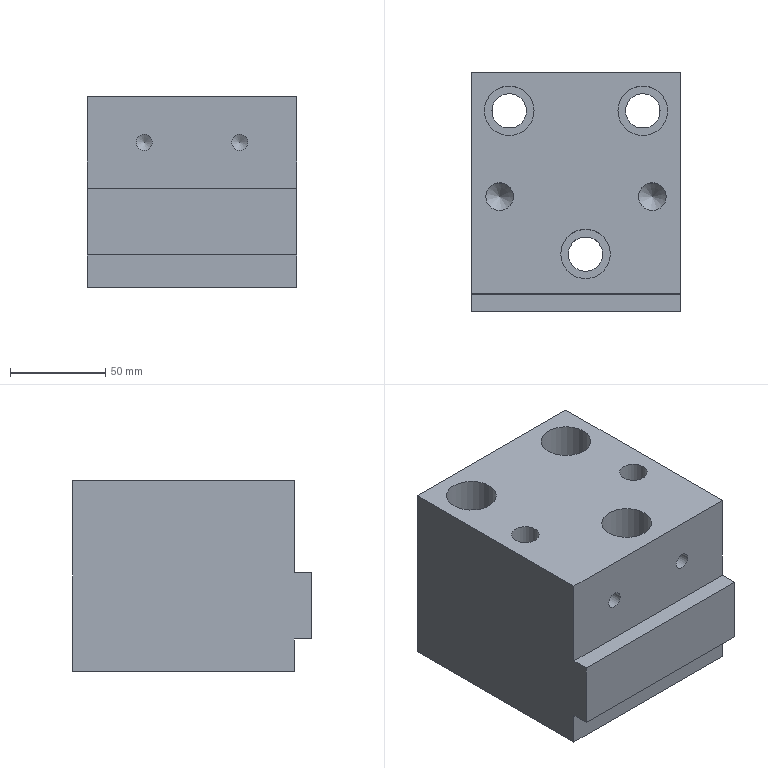Part | STEP file | lll_id4734_x_t | 1 solid | 27 faces | box 110 x 125 x 100 mm | volume 1168907 mm3 | plane 13 | cylinder 10 | cone 4 | commonest cylinder face diameters 18.009 x3 26.008 x3 8.5 x2 14.506 x2
STEP:
#1=CARTESIAN_POINT('',(1322.592,417.359,5.));
#2=VERTEX_POINT('',#1);
#3=CARTESIAN_POINT('',(1315.339,417.359,5.));
#4=DIRECTION('',(0.,0.,-1.));
#5=DIRECTION('',(1.,0.,0.));
#6=AXIS2_PLACEMENT_3D('',#3,#4,#5);
#7=CIRCLE('',#6,7.253);
#8=EDGE_CURVE('',#2,#2,#7,.T.);
#9=ORIENTED_EDGE('',*,*,#8,.T.);
#10=EDGE_LOOP('',(#9));
#11=FACE_BOUND('',#10,.T.);
#12=CARTESIAN_POINT('',(1402.592,417.359,5.));
#13=VERTEX_POINT('',#12);
#14=CARTESIAN_POINT('',(1395.339,417.359,5.));
#15=DIRECTION('',(0.,0.,-1.));
#16=DIRECTION('',(1.,0.,0.));
#17=AXIS2_PLACEMENT_3D('',#14,#15,#16);
#18=CIRCLE('',#17,7.253);
#19=EDGE_CURVE('',#13,#13,#18,.T.);
#20=ORIENTED_EDGE('',*,*,#19,.T.);
#21=EDGE_LOOP('',(#20));
#22=FACE_BOUND('',#21,.T.);
#23=CARTESIAN_POINT('',(1300.339,366.359,5.));
#24=VERTEX_POINT('',#23);
#25=CARTESIAN_POINT('',(1410.339,366.359,5.));
#26=VERTEX_POINT('',#25);
#27=CARTESIAN_POINT('',(-3297.001,366.359,5.));
#28=DIRECTION('',(1.,0.,0.));
#29=VECTOR('',#28,1.);
#30=LINE('',#27,#29);
#31=EDGE_CURVE('',#24,#26,#30,.T.);
#32=ORIENTED_EDGE('',*,*,#31,.T.);
#33=CARTESIAN_POINT('',(1410.339,482.359,5.));
#34=VERTEX_POINT('',#33);
#35=CARTESIAN_POINT('',(1410.339,382.359,5.));
#36=DIRECTION('',(0.,-1.,0.));
#37=VECTOR('',#36,1.);
#38=LINE('',#35,#37);
#39=EDGE_CURVE('',#34,#26,#38,.T.);
#40=ORIENTED_EDGE('',*,*,#39,.F.);
#41=CARTESIAN_POINT('',(1300.339,482.359,5.));
#42=VERTEX_POINT('',#41);
#43=CARTESIAN_POINT('',(1308.588,482.359,5.));
#44=DIRECTION('',(-1.,0.,0.));
#45=VECTOR('',#44,1.);
#46=LINE('',#43,#45);
#47=EDGE_CURVE('',#34,#42,#46,.T.);
#48=ORIENTED_EDGE('',*,*,#47,.T.);
#49=CARTESIAN_POINT('',(1300.339,382.359,5.));
#50=DIRECTION('',(0.,1.,0.));
#51=VECTOR('',#50,1.);
#52=LINE('',#49,#51);
#53=EDGE_CURVE('',#24,#42,#52,.T.);
#54=ORIENTED_EDGE('',*,*,#53,.F.);
#55=EDGE_LOOP('',(#32,#40,#48,#54));
#56=FACE_BOUND('',#55,.T.);
#57=CARTESIAN_POINT('',(1377.335,462.359,5.));
#58=VERTEX_POINT('',#57);
#59=CARTESIAN_POINT('',(1390.339,462.359,5.));
#60=DIRECTION('',(0.,0.,-1.));
#61=DIRECTION('',(-1.,0.,0.));
#62=AXIS2_PLACEMENT_3D('',#59,#60,#61);
#63=CIRCLE('',#62,13.004);
#64=EDGE_CURVE('',#58,#58,#63,.T.);
#65=ORIENTED_EDGE('',*,*,#64,.T.);
#66=EDGE_LOOP('',(#65));
#67=FACE_BOUND('',#66,.T.);
#68=CARTESIAN_POINT('',(1307.335,462.359,5.));
#69=VERTEX_POINT('',#68);
#70=CARTESIAN_POINT('',(1320.339,462.359,5.));
#71=DIRECTION('',(0.,0.,-1.));
#72=DIRECTION('',(-1.,0.,0.));
#73=AXIS2_PLACEMENT_3D('',#70,#71,#72);
#74=CIRCLE('',#73,13.004);
#75=EDGE_CURVE('',#69,#69,#74,.T.);
#76=ORIENTED_EDGE('',*,*,#75,.T.);
#77=EDGE_LOOP('',(#76));
#78=FACE_BOUND('',#77,.T.);
#79=CARTESIAN_POINT('',(1373.343,387.359,5.));
#80=VERTEX_POINT('',#79);
#81=CARTESIAN_POINT('',(1360.339,387.359,5.));
#82=DIRECTION('',(0.,0.,1.));
#83=DIRECTION('',(1.,0.,0.));
#84=AXIS2_PLACEMENT_3D('',#81,#82,#83);
#85=CIRCLE('',#84,13.004);
#86=EDGE_CURVE('',#80,#80,#85,.T.);
#87=ORIENTED_EDGE('',*,*,#86,.F.);
#88=EDGE_LOOP('',(#87));
#89=FACE_BOUND('',#88,.T.);
#90=CARTESIAN_POINT('',(1308.588,382.359,5.));
#91=DIRECTION('',(0.,0.,-1.));
#92=DIRECTION('',(1.,0.,0.));
#93=AXIS2_PLACEMENT_3D('',#90,#91,#92);
#94=PLANE('',#93);
#95=ADVANCED_FACE('',(#11,#22,#56,#67,#78,#89),#94,.F.);
#96=CARTESIAN_POINT('',(1330.339,366.359,-23.25));
#97=VERTEX_POINT('',#96);
#98=CARTESIAN_POINT('',(1330.339,366.359,-19.));
#99=DIRECTION('',(0.,-1.,0.));
#100=DIRECTION('',(0.,0.,-1.));
#101=AXIS2_PLACEMENT_3D('',#98,#99,#100);
#102=CIRCLE('',#101,4.25);
#103=EDGE_CURVE('',#97,#97,#102,.T.);
#104=ORIENTED_EDGE('',*,*,#103,.F.);
#105=EDGE_LOOP('',(#104));
#106=FACE_BOUND('',#105,.T.);
#107=CARTESIAN_POINT('',(1380.339,366.359,-23.25));
#108=VERTEX_POINT('',#107);
#109=CARTESIAN_POINT('',(1380.339,366.359,-19.));
#110=DIRECTION('',(0.,-1.,0.));
#111=DIRECTION('',(0.,0.,-1.));
#112=AXIS2_PLACEMENT_3D('',#109,#110,#111);
#113=CIRCLE('',#112,4.25);
#114=EDGE_CURVE('',#108,#108,#113,.T.);
#115=ORIENTED_EDGE('',*,*,#114,.F.);
#116=EDGE_LOOP('',(#115));
#117=FACE_BOUND('',#116,.T.);
#118=CARTESIAN_POINT('',(1300.339,366.359,-43.));
#119=VERTEX_POINT('',#118);
#120=CARTESIAN_POINT('',(1410.339,366.359,-43.));
#121=VERTEX_POINT('',#120);
#122=CARTESIAN_POINT('',(1305.339,366.359,-43.));
#123=DIRECTION('',(1.,0.,0.));
#124=VECTOR('',#123,1.);
#125=LINE('',#122,#124);
#126=EDGE_CURVE('',#119,#121,#125,.T.);
#127=ORIENTED_EDGE('',*,*,#126,.T.);
#128=CARTESIAN_POINT('',(1410.339,366.359,-35.));
#129=DIRECTION('',(0.,0.,1.));
#130=VECTOR('',#129,1.);
#131=LINE('',#128,#130);
#132=EDGE_CURVE('',#121,#26,#131,.T.);
#133=ORIENTED_EDGE('',*,*,#132,.T.);
#134=ORIENTED_EDGE('',*,*,#31,.F.);
#135=CARTESIAN_POINT('',(1300.339,366.359,-625.));
#136=DIRECTION('',(0.,0.,-1.));
#137=VECTOR('',#136,1.);
#138=LINE('',#135,#137);
#139=EDGE_CURVE('',#24,#119,#138,.T.);
#140=ORIENTED_EDGE('',*,*,#139,.T.);
#141=EDGE_LOOP('',(#127,#133,#134,#140));
#142=FACE_BOUND('',#141,.T.);
#143=CARTESIAN_POINT('',(-3297.001,366.359,-625.));
#144=DIRECTION('',(0.,-1.,0.));
#145=DIRECTION('',(0.,0.,1.));
#146=AXIS2_PLACEMENT_3D('',#143,#144,#145);
#147=PLANE('',#146);
#148=ADVANCED_FACE('',(#106,#117,#142),#147,.T.);
#149=CARTESIAN_POINT('',(1300.339,482.359,-95.));
#150=VERTEX_POINT('',#149);
#151=CARTESIAN_POINT('',(1300.339,482.359,-650.));
#152=DIRECTION('',(0.,0.,-1.));
#153=VECTOR('',#152,1.);
#154=LINE('',#151,#153);
#155=EDGE_CURVE('',#42,#150,#154,.T.);
#156=ORIENTED_EDGE('',*,*,#155,.T.);
#157=CARTESIAN_POINT('',(1300.339,366.359,-95.));
#158=VERTEX_POINT('',#157);
#159=CARTESIAN_POINT('',(1300.339,407.359,-95.));
#160=DIRECTION('',(0.,-1.,0.));
#161=VECTOR('',#160,1.);
#162=LINE('',#159,#161);
#163=EDGE_CURVE('',#150,#158,#162,.T.);
#164=ORIENTED_EDGE('',*,*,#163,.T.);
#165=CARTESIAN_POINT('',(1300.339,366.359,-78.));
#166=VERTEX_POINT('',#165);
#167=CARTESIAN_POINT('',(1300.339,366.359,-625.));
#168=DIRECTION('',(0.,0.,-1.));
#169=VECTOR('',#168,1.);
#170=LINE('',#167,#169);
#171=EDGE_CURVE('',#166,#158,#170,.T.);
#172=ORIENTED_EDGE('',*,*,#171,.F.);
#173=CARTESIAN_POINT('',(1300.339,357.359,-78.));
#174=VERTEX_POINT('',#173);
#175=CARTESIAN_POINT('',(1300.339,407.359,-78.));
#176=DIRECTION('',(0.,-1.,0.));
#177=VECTOR('',#176,1.);
#178=LINE('',#175,#177);
#179=EDGE_CURVE('',#166,#174,#178,.T.);
#180=ORIENTED_EDGE('',*,*,#179,.T.);
#181=CARTESIAN_POINT('',(1300.339,357.359,-43.));
#182=VERTEX_POINT('',#181);
#183=CARTESIAN_POINT('',(1300.339,357.359,72.5));
#184=DIRECTION('',(0.,0.,-1.));
#185=VECTOR('',#184,1.);
#186=LINE('',#183,#185);
#187=EDGE_CURVE('',#182,#174,#186,.T.);
#188=ORIENTED_EDGE('',*,*,#187,.F.);
#189=CARTESIAN_POINT('',(1300.339,397.359,-43.));
#190=DIRECTION('',(0.,-1.,0.));
#191=VECTOR('',#190,1.);
#192=LINE('',#189,#191);
#193=EDGE_CURVE('',#119,#182,#192,.T.);
#194=ORIENTED_EDGE('',*,*,#193,.F.);
#195=ORIENTED_EDGE('',*,*,#139,.F.);
#196=ORIENTED_EDGE('',*,*,#53,.T.);
#197=EDGE_LOOP('',(#156,#164,#172,#180,#188,#194,#195,#196));
#198=FACE_OUTER_BOUND('',#197,.T.);
#199=CARTESIAN_POINT('',(1300.339,407.359,72.5));
#200=DIRECTION('',(-1.,0.,0.));
#201=DIRECTION('',(0.,0.,-1.));
#202=AXIS2_PLACEMENT_3D('',#199,#200,#201);
#203=PLANE('',#202);
#204=ADVANCED_FACE('',(#198),#203,.T.);
#205=CARTESIAN_POINT('',(1410.339,357.359,-78.));
#206=VERTEX_POINT('',#205);
#207=CARTESIAN_POINT('',(-3297.001,357.359,-78.));
#208=DIRECTION('',(-1.,0.,0.));
#209=VECTOR('',#208,1.);
#210=LINE('',#207,#209);
#211=EDGE_CURVE('',#206,#174,#210,.T.);
#212=ORIENTED_EDGE('',*,*,#211,.F.);
#213=CARTESIAN_POINT('',(1410.339,357.359,-43.));
#214=VERTEX_POINT('',#213);
#215=CARTESIAN_POINT('',(1410.339,357.359,-60.));
#216=DIRECTION('',(0.,0.,1.));
#217=VECTOR('',#216,1.);
#218=LINE('',#215,#217);
#219=EDGE_CURVE('',#206,#214,#218,.T.);
#220=ORIENTED_EDGE('',*,*,#219,.T.);
#221=CARTESIAN_POINT('',(-3297.001,357.359,-43.));
#222=DIRECTION('',(-1.,0.,0.));
#223=VECTOR('',#222,1.);
#224=LINE('',#221,#223);
#225=EDGE_CURVE('',#214,#182,#224,.T.);
#226=ORIENTED_EDGE('',*,*,#225,.T.);
#227=ORIENTED_EDGE('',*,*,#187,.T.);
#228=EDGE_LOOP('',(#212,#220,#226,#227));
#229=FACE_OUTER_BOUND('',#228,.T.);
#230=CARTESIAN_POINT('',(-3297.001,357.359,-650.));
#231=DIRECTION('',(0.,-1.,0.));
#232=DIRECTION('',(0.,0.,1.));
#233=AXIS2_PLACEMENT_3D('',#230,#231,#232);
#234=PLANE('',#233);
#235=ADVANCED_FACE('',(#229),#234,.T.);
#236=CARTESIAN_POINT('',(1410.339,482.359,-95.));
#237=VERTEX_POINT('',#236);
#238=CARTESIAN_POINT('',(1410.339,482.359,-650.));
#239=DIRECTION('',(0.,0.,-1.));
#240=VECTOR('',#239,1.);
#241=LINE('',#238,#240);
#242=EDGE_CURVE('',#34,#237,#241,.T.);
#243=ORIENTED_EDGE('',*,*,#242,.T.);
#244=CARTESIAN_POINT('',(-3297.001,482.359,-95.));
#245=DIRECTION('',(1.,0.,0.));
#246=VECTOR('',#245,1.);
#247=LINE('',#244,#246);
#248=EDGE_CURVE('',#150,#237,#247,.T.);
#249=ORIENTED_EDGE('',*,*,#248,.F.);
#250=ORIENTED_EDGE('',*,*,#155,.F.);
#251=ORIENTED_EDGE('',*,*,#47,.F.);
#252=EDGE_LOOP('',(#243,#249,#250,#251));
#253=FACE_OUTER_BOUND('',#252,.T.);
#254=CARTESIAN_POINT('',(-3297.001,482.359,-650.));
#255=DIRECTION('',(0.,-1.,0.));
#256=DIRECTION('',(0.,0.,1.));
#257=AXIS2_PLACEMENT_3D('',#254,#255,#256);
#258=PLANE('',#257);
#259=ADVANCED_FACE('',(#253),#258,.F.);
#260=ORIENTED_EDGE('',*,*,#219,.F.);
#261=CARTESIAN_POINT('',(1410.339,366.359,-78.));
#262=VERTEX_POINT('',#261);
#263=CARTESIAN_POINT('',(1410.339,382.359,-78.));
#264=DIRECTION('',(0.,-1.,0.));
#265=VECTOR('',#264,1.);
#266=LINE('',#263,#265);
#267=EDGE_CURVE('',#262,#206,#266,.T.);
#268=ORIENTED_EDGE('',*,*,#267,.F.);
#269=CARTESIAN_POINT('',(1410.339,366.359,-95.));
#270=VERTEX_POINT('',#269);
#271=CARTESIAN_POINT('',(1410.339,366.359,-60.));
#272=DIRECTION('',(0.,0.,1.));
#273=VECTOR('',#272,1.);
#274=LINE('',#271,#273);
#275=EDGE_CURVE('',#270,#262,#274,.T.);
#276=ORIENTED_EDGE('',*,*,#275,.F.);
#277=CARTESIAN_POINT('',(1410.339,233.52,-95.));
#278=DIRECTION('',(0.,1.,0.));
#279=VECTOR('',#278,1.);
#280=LINE('',#277,#279);
#281=EDGE_CURVE('',#270,#237,#280,.T.);
#282=ORIENTED_EDGE('',*,*,#281,.T.);
#283=ORIENTED_EDGE('',*,*,#242,.F.);
#284=ORIENTED_EDGE('',*,*,#39,.T.);
#285=ORIENTED_EDGE('',*,*,#132,.F.);
#286=CARTESIAN_POINT('',(1410.339,382.359,-43.));
#287=DIRECTION('',(0.,1.,0.));
#288=VECTOR('',#287,1.);
#289=LINE('',#286,#288);
#290=EDGE_CURVE('',#214,#121,#289,.T.);
#291=ORIENTED_EDGE('',*,*,#290,.F.);
#292=EDGE_LOOP('',(#260,#268,#276,#282,#283,#284,#285,#291));
#293=FACE_OUTER_BOUND('',#292,.T.);
#294=CARTESIAN_POINT('',(1410.339,382.359,-60.));
#295=DIRECTION('',(-1.,0.,0.));
#296=DIRECTION('',(0.,0.,-1.));
#297=AXIS2_PLACEMENT_3D('',#294,#295,#296);
#298=PLANE('',#297);
#299=ADVANCED_FACE('',(#293),#298,.F.);
#300=ORIENTED_EDGE('',*,*,#126,.F.);
#301=ORIENTED_EDGE('',*,*,#193,.T.);
#302=ORIENTED_EDGE('',*,*,#225,.F.);
#303=ORIENTED_EDGE('',*,*,#290,.T.);
#304=EDGE_LOOP('',(#300,#301,#302,#303));
#305=FACE_OUTER_BOUND('',#304,.T.);
#306=CARTESIAN_POINT('',(1305.339,397.359,-43.));
#307=DIRECTION('',(0.,0.,1.));
#308=DIRECTION('',(-1.,0.,0.));
#309=AXIS2_PLACEMENT_3D('',#306,#307,#308);
#310=PLANE('',#309);
#311=ADVANCED_FACE('',(#305),#310,.T.);
#312=CARTESIAN_POINT('',(1399.344,462.359,-55.));
#313=VERTEX_POINT('',#312);
#314=CARTESIAN_POINT('',(1390.339,462.359,-55.));
#315=DIRECTION('',(0.,0.,-1.));
#316=DIRECTION('',(1.,0.,0.));
#317=AXIS2_PLACEMENT_3D('',#314,#315,#316);
#318=CIRCLE('',#317,9.005);
#319=EDGE_CURVE('',#313,#313,#318,.T.);
#320=ORIENTED_EDGE('',*,*,#319,.F.);
#321=EDGE_LOOP('',(#320));
#322=FACE_BOUND('',#321,.T.);
#323=CARTESIAN_POINT('',(1399.344,462.359,-95.));
#324=VERTEX_POINT('',#323);
#325=CARTESIAN_POINT('',(1390.339,462.359,-95.));
#326=DIRECTION('',(0.,0.,-1.));
#327=DIRECTION('',(1.,0.,0.));
#328=AXIS2_PLACEMENT_3D('',#325,#326,#327);
#329=CIRCLE('',#328,9.005);
#330=EDGE_CURVE('',#324,#324,#329,.T.);
#331=ORIENTED_EDGE('',*,*,#330,.T.);
#332=EDGE_LOOP('',(#331));
#333=FACE_BOUND('',#332,.T.);
#334=CARTESIAN_POINT('',(1390.339,462.359,-18.));
#335=DIRECTION('',(0.,0.,-1.));
#336=DIRECTION('',(-1.,0.,0.));
#337=AXIS2_PLACEMENT_3D('',#334,#335,#336);
#338=CYLINDRICAL_SURFACE('',#337,9.005);
#339=ADVANCED_FACE('',(#322,#333),#338,.F.);
#340=ORIENTED_EDGE('',*,*,#319,.T.);
#341=EDGE_LOOP('',(#340));
#342=FACE_BOUND('',#341,.T.);
#343=CARTESIAN_POINT('',(1377.335,462.359,-55.));
#344=VERTEX_POINT('',#343);
#345=CARTESIAN_POINT('',(1390.339,462.359,-55.));
#346=DIRECTION('',(0.,0.,-1.));
#347=DIRECTION('',(-1.,0.,0.));
#348=AXIS2_PLACEMENT_3D('',#345,#346,#347);
#349=CIRCLE('',#348,13.004);
#350=EDGE_CURVE('',#344,#344,#349,.T.);
#351=ORIENTED_EDGE('',*,*,#350,.F.);
#352=EDGE_LOOP('',(#351));
#353=FACE_BOUND('',#352,.T.);
#354=CARTESIAN_POINT('',(1390.339,462.359,-55.));
#355=DIRECTION('',(0.,0.,-1.));
#356=DIRECTION('',(1.,0.,0.));
#357=AXIS2_PLACEMENT_3D('',#354,#355,#356);
#358=PLANE('',#357);
#359=ADVANCED_FACE('',(#342,#353),#358,.F.);
#360=ORIENTED_EDGE('',*,*,#350,.T.);
#361=EDGE_LOOP('',(#360));
#362=FACE_BOUND('',#361,.T.);
#363=ORIENTED_EDGE('',*,*,#64,.F.);
#364=EDGE_LOOP('',(#363));
#365=FACE_BOUND('',#364,.T.);
#366=CARTESIAN_POINT('',(1390.339,462.359,5.));
#367=DIRECTION('',(0.,0.,-1.));
#368=DIRECTION('',(-1.,0.,0.));
#369=AXIS2_PLACEMENT_3D('',#366,#367,#368);
#370=CYLINDRICAL_SURFACE('',#369,13.004);
#371=ADVANCED_FACE('',(#362,#365),#370,.F.);
#372=CARTESIAN_POINT('',(1329.344,462.359,-55.));
#373=VERTEX_POINT('',#372);
#374=CARTESIAN_POINT('',(1320.339,462.359,-55.));
#375=DIRECTION('',(0.,0.,-1.));
#376=DIRECTION('',(0.,1.,0.));
#377=AXIS2_PLACEMENT_3D('',#374,#375,#376);
#378=CIRCLE('',#377,9.005);
#379=EDGE_CURVE('',#373,#373,#378,.T.);
#380=ORIENTED_EDGE('',*,*,#379,.F.);
#381=EDGE_LOOP('',(#380));
#382=FACE_BOUND('',#381,.T.);
#383=CARTESIAN_POINT('',(1329.344,462.359,-95.));
#384=VERTEX_POINT('',#383);
#385=CARTESIAN_POINT('',(1320.339,462.359,-95.));
#386=DIRECTION('',(0.,0.,-1.));
#387=DIRECTION('',(1.,0.,0.));
#388=AXIS2_PLACEMENT_3D('',#385,#386,#387);
#389=CIRCLE('',#388,9.005);
#390=EDGE_CURVE('',#384,#384,#389,.T.);
#391=ORIENTED_EDGE('',*,*,#390,.T.);
#392=EDGE_LOOP('',(#391));
#393=FACE_BOUND('',#392,.T.);
#394=CARTESIAN_POINT('',(1320.339,462.359,-18.));
#395=DIRECTION('',(0.,0.,-1.));
#396=DIRECTION('',(-1.,0.,0.));
#397=AXIS2_PLACEMENT_3D('',#394,#395,#396);
#398=CYLINDRICAL_SURFACE('',#397,9.005);
#399=ADVANCED_FACE('',(#382,#393),#398,.F.);
#400=ORIENTED_EDGE('',*,*,#379,.T.);
#401=EDGE_LOOP('',(#400));
#402=FACE_BOUND('',#401,.T.);
#403=CARTESIAN_POINT('',(1307.335,462.359,-55.));
#404=VERTEX_POINT('',#403);
#405=CARTESIAN_POINT('',(1320.339,462.359,-55.));
#406=DIRECTION('',(0.,0.,-1.));
#407=DIRECTION('',(0.,1.,0.));
#408=AXIS2_PLACEMENT_3D('',#405,#406,#407);
#409=CIRCLE('',#408,13.004);
#410=EDGE_CURVE('',#404,#404,#409,.T.);
#411=ORIENTED_EDGE('',*,*,#410,.F.);
#412=EDGE_LOOP('',(#411));
#413=FACE_BOUND('',#412,.T.);
#414=CARTESIAN_POINT('',(1320.339,462.359,-55.));
#415=DIRECTION('',(0.,0.,-1.));
#416=DIRECTION('',(1.,0.,0.));
#417=AXIS2_PLACEMENT_3D('',#414,#415,#416);
#418=PLANE('',#417);
#419=ADVANCED_FACE('',(#402,#413),#418,.F.);
#420=ORIENTED_EDGE('',*,*,#410,.T.);
#421=EDGE_LOOP('',(#420));
#422=FACE_BOUND('',#421,.T.);
#423=ORIENTED_EDGE('',*,*,#75,.F.);
#424=EDGE_LOOP('',(#423));
#425=FACE_BOUND('',#424,.T.);
#426=CARTESIAN_POINT('',(1320.339,462.359,5.));
#427=DIRECTION('',(0.,0.,-1.));
#428=DIRECTION('',(-1.,0.,0.));
#429=AXIS2_PLACEMENT_3D('',#426,#427,#428);
#430=CYLINDRICAL_SURFACE('',#429,13.004);
#431=ADVANCED_FACE('',(#422,#425),#430,.F.);
#432=CARTESIAN_POINT('',(1351.335,387.359,-55.));
#433=VERTEX_POINT('',#432);
#434=CARTESIAN_POINT('',(1360.339,387.359,-55.));
#435=DIRECTION('',(0.,0.,1.));
#436=DIRECTION('',(-1.,0.,0.));
#437=AXIS2_PLACEMENT_3D('',#434,#435,#436);
#438=CIRCLE('',#437,9.005);
#439=EDGE_CURVE('',#433,#433,#438,.T.);
#440=ORIENTED_EDGE('',*,*,#439,.T.);
#441=EDGE_LOOP('',(#440));
#442=FACE_BOUND('',#441,.T.);
#443=CARTESIAN_POINT('',(1369.344,387.359,-95.));
#444=VERTEX_POINT('',#443);
#445=CARTESIAN_POINT('',(1360.339,387.359,-95.));
#446=DIRECTION('',(0.,0.,-1.));
#447=DIRECTION('',(1.,0.,0.));
#448=AXIS2_PLACEMENT_3D('',#445,#446,#447);
#449=CIRCLE('',#448,9.005);
#450=EDGE_CURVE('',#444,#444,#449,.T.);
#451=ORIENTED_EDGE('',*,*,#450,.T.);
#452=EDGE_LOOP('',(#451));
#453=FACE_BOUND('',#452,.T.);
#454=CARTESIAN_POINT('',(1360.339,387.359,-18.));
#455=DIRECTION('',(0.,0.,-1.));
#456=DIRECTION('',(1.,0.,0.));
#457=AXIS2_PLACEMENT_3D('',#454,#455,#456);
#458=CYLINDRICAL_SURFACE('',#457,9.005);
#459=ADVANCED_FACE('',(#442,#453),#458,.F.);
#460=ORIENTED_EDGE('',*,*,#439,.F.);
#461=EDGE_LOOP('',(#460));
#462=FACE_BOUND('',#461,.T.);
#463=CARTESIAN_POINT('',(1373.343,387.359,-55.));
#464=VERTEX_POINT('',#463);
#465=CARTESIAN_POINT('',(1360.339,387.359,-55.));
#466=DIRECTION('',(0.,0.,1.));
#467=DIRECTION('',(1.,0.,0.));
#468=AXIS2_PLACEMENT_3D('',#465,#466,#467);
#469=CIRCLE('',#468,13.004);
#470=EDGE_CURVE('',#464,#464,#469,.T.);
#471=ORIENTED_EDGE('',*,*,#470,.T.);
#472=EDGE_LOOP('',(#471));
#473=FACE_BOUND('',#472,.T.);
#474=CARTESIAN_POINT('',(1360.339,387.359,-55.));
#475=DIRECTION('',(0.,0.,-1.));
#476=DIRECTION('',(-1.,0.,0.));
#477=AXIS2_PLACEMENT_3D('',#474,#475,#476);
#478=PLANE('',#477);
#479=ADVANCED_FACE('',(#462,#473),#478,.F.);
#480=ORIENTED_EDGE('',*,*,#470,.F.);
#481=EDGE_LOOP('',(#480));
#482=FACE_BOUND('',#481,.T.);
#483=ORIENTED_EDGE('',*,*,#86,.T.);
#484=EDGE_LOOP('',(#483));
#485=FACE_BOUND('',#484,.T.);
#486=CARTESIAN_POINT('',(1360.339,387.359,5.));
#487=DIRECTION('',(0.,0.,-1.));
#488=DIRECTION('',(1.,0.,0.));
#489=AXIS2_PLACEMENT_3D('',#486,#487,#488);
#490=CYLINDRICAL_SURFACE('',#489,13.004);
#491=ADVANCED_FACE('',(#482,#485),#490,.F.);
#492=CARTESIAN_POINT('',(1402.592,417.359,-30.753));
#493=VERTEX_POINT('',#492);
#494=CARTESIAN_POINT('',(1395.339,417.359,-30.753));
#495=DIRECTION('',(0.,0.,-1.));
#496=DIRECTION('',(1.,0.,0.));
#497=AXIS2_PLACEMENT_3D('',#494,#495,#496);
#498=CIRCLE('',#497,7.253);
#499=EDGE_CURVE('',#493,#493,#498,.T.);
#500=ORIENTED_EDGE('',*,*,#499,.T.);
#501=EDGE_LOOP('',(#500));
#502=FACE_BOUND('',#501,.T.);
#503=ORIENTED_EDGE('',*,*,#19,.F.);
#504=EDGE_LOOP('',(#503));
#505=FACE_BOUND('',#504,.T.);
#506=CARTESIAN_POINT('',(1395.339,417.359,7.));
#507=DIRECTION('',(0.,0.,-1.));
#508=DIRECTION('',(-1.,0.,0.));
#509=AXIS2_PLACEMENT_3D('',#506,#507,#508);
#510=CYLINDRICAL_SURFACE('',#509,7.253);
#511=ADVANCED_FACE('',(#502,#505),#510,.F.);
#512=CARTESIAN_POINT('',(1395.339,417.359,-38.006));
#513=VERTEX_POINT('',#512);
#514=VERTEX_LOOP('',#513);
#515=FACE_BOUND('',#514,.T.);
#516=ORIENTED_EDGE('',*,*,#499,.F.);
#517=EDGE_LOOP('',(#516));
#518=FACE_BOUND('',#517,.T.);
#519=CARTESIAN_POINT('',(1395.339,417.359,-30.753));
#520=DIRECTION('',(0.,0.,1.));
#521=DIRECTION('',(-1.,0.,0.));
#522=AXIS2_PLACEMENT_3D('',#519,#520,#521);
#523=CONICAL_SURFACE('',#522,7.253,45.);
#524=ADVANCED_FACE('',(#515,#518),#523,.F.);
#525=CARTESIAN_POINT('',(1308.086,417.359,-30.753));
#526=VERTEX_POINT('',#525);
#527=CARTESIAN_POINT('',(1315.339,417.359,-30.753));
#528=DIRECTION('',(0.,0.,1.));
#529=DIRECTION('',(-1.,0.,0.));
#530=AXIS2_PLACEMENT_3D('',#527,#528,#529);
#531=CIRCLE('',#530,7.253);
#532=EDGE_CURVE('',#526,#526,#531,.T.);
#533=ORIENTED_EDGE('',*,*,#532,.F.);
#534=EDGE_LOOP('',(#533));
#535=FACE_BOUND('',#534,.T.);
#536=ORIENTED_EDGE('',*,*,#8,.F.);
#537=EDGE_LOOP('',(#536));
#538=FACE_BOUND('',#537,.T.);
#539=CARTESIAN_POINT('',(1315.339,417.359,7.));
#540=DIRECTION('',(0.,0.,-1.));
#541=DIRECTION('',(1.,0.,0.));
#542=AXIS2_PLACEMENT_3D('',#539,#540,#541);
#543=CYLINDRICAL_SURFACE('',#542,7.253);
#544=ADVANCED_FACE('',(#535,#538),#543,.F.);
#545=CARTESIAN_POINT('',(1315.339,417.359,-38.006));
#546=VERTEX_POINT('',#545);
#547=VERTEX_LOOP('',#546);
#548=FACE_BOUND('',#547,.T.);
#549=ORIENTED_EDGE('',*,*,#532,.T.);
#550=EDGE_LOOP('',(#549));
#551=FACE_BOUND('',#550,.T.);
#552=CARTESIAN_POINT('',(1315.339,417.359,-30.753));
#553=DIRECTION('',(0.,0.,1.));
#554=DIRECTION('',(1.,0.,0.));
#555=AXIS2_PLACEMENT_3D('',#552,#553,#554);
#556=CONICAL_SURFACE('',#555,7.253,45.);
#557=ADVANCED_FACE('',(#548,#551),#556,.F.);
#558=CARTESIAN_POINT('',(1380.339,396.359,-23.25));
#559=VERTEX_POINT('',#558);
#560=CARTESIAN_POINT('',(1380.339,396.359,-19.));
#561=DIRECTION('',(0.,1.,0.));
#562=DIRECTION('',(0.,0.,-1.));
#563=AXIS2_PLACEMENT_3D('',#560,#561,#562);
#564=CIRCLE('',#563,4.25);
#565=EDGE_CURVE('',#559,#559,#564,.T.);
#566=ORIENTED_EDGE('',*,*,#565,.F.);
#567=EDGE_LOOP('',(#566));
#568=FACE_BOUND('',#567,.T.);
#569=CARTESIAN_POINT('',(1380.339,398.913,-19.));
#570=VERTEX_POINT('',#569);
#571=VERTEX_LOOP('',#570);
#572=FACE_BOUND('',#571,.T.);
#573=CARTESIAN_POINT('',(1380.339,396.359,-19.));
#574=DIRECTION('',(0.,-1.,0.));
#575=DIRECTION('',(0.,0.,1.));
#576=AXIS2_PLACEMENT_3D('',#573,#574,#575);
#577=CONICAL_SURFACE('',#576,4.25,59.);
#578=ADVANCED_FACE('',(#568,#572),#577,.F.);
#579=ORIENTED_EDGE('',*,*,#565,.T.);
#580=EDGE_LOOP('',(#579));
#581=FACE_BOUND('',#580,.T.);
#582=ORIENTED_EDGE('',*,*,#114,.T.);
#583=EDGE_LOOP('',(#582));
#584=FACE_BOUND('',#583,.T.);
#585=CARTESIAN_POINT('',(1380.339,366.359,-19.));
#586=DIRECTION('',(0.,1.,0.));
#587=DIRECTION('',(0.,0.,-1.));
#588=AXIS2_PLACEMENT_3D('',#585,#586,#587);
#589=CYLINDRICAL_SURFACE('',#588,4.25);
#590=ADVANCED_FACE('',(#581,#584),#589,.F.);
#591=CARTESIAN_POINT('',(1330.339,386.359,-23.25));
#592=VERTEX_POINT('',#591);
#593=CARTESIAN_POINT('',(1330.339,386.359,-19.));
#594=DIRECTION('',(0.,1.,0.));
#595=DIRECTION('',(0.,0.,-1.));
#596=AXIS2_PLACEMENT_3D('',#593,#594,#595);
#597=CIRCLE('',#596,4.25);
#598=EDGE_CURVE('',#592,#592,#597,.T.);
#599=ORIENTED_EDGE('',*,*,#598,.F.);
#600=EDGE_LOOP('',(#599));
#601=FACE_BOUND('',#600,.T.);
#602=CARTESIAN_POINT('',(1330.339,388.913,-19.));
#603=VERTEX_POINT('',#602);
#604=VERTEX_LOOP('',#603);
#605=FACE_BOUND('',#604,.T.);
#606=CARTESIAN_POINT('',(1330.339,386.359,-19.));
#607=DIRECTION('',(0.,-1.,0.));
#608=DIRECTION('',(0.,0.,1.));
#609=AXIS2_PLACEMENT_3D('',#606,#607,#608);
#610=CONICAL_SURFACE('',#609,4.25,59.);
#611=ADVANCED_FACE('',(#601,#605),#610,.F.);
#612=ORIENTED_EDGE('',*,*,#598,.T.);
#613=EDGE_LOOP('',(#612));
#614=FACE_BOUND('',#613,.T.);
#615=ORIENTED_EDGE('',*,*,#103,.T.);
#616=EDGE_LOOP('',(#615));
#617=FACE_BOUND('',#616,.T.);
#618=CARTESIAN_POINT('',(1330.339,366.359,-19.));
#619=DIRECTION('',(0.,1.,0.));
#620=DIRECTION('',(0.,0.,-1.));
#621=AXIS2_PLACEMENT_3D('',#618,#619,#620);
#622=CYLINDRICAL_SURFACE('',#621,4.25);
#623=ADVANCED_FACE('',(#614,#617),#622,.F.);
#624=ORIENTED_EDGE('',*,*,#179,.F.);
#625=CARTESIAN_POINT('',(2067.435,366.359,-78.));
#626=DIRECTION('',(1.,0.,0.));
#627=VECTOR('',#626,1.);
#628=LINE('',#625,#627);
#629=EDGE_CURVE('',#166,#262,#628,.T.);
#630=ORIENTED_EDGE('',*,*,#629,.T.);
#631=ORIENTED_EDGE('',*,*,#267,.T.);
#632=ORIENTED_EDGE('',*,*,#211,.T.);
#633=EDGE_LOOP('',(#624,#630,#631,#632));
#634=FACE_OUTER_BOUND('',#633,.T.);
#635=CARTESIAN_POINT('',(2067.435,0.000000688,-78.));
#636=DIRECTION('',(0.,0.,1.));
#637=DIRECTION('',(-1.,0.,0.));
#638=AXIS2_PLACEMENT_3D('',#635,#636,#637);
#639=PLANE('',#638);
#640=ADVANCED_FACE('',(#634),#639,.F.);
#641=ORIENTED_EDGE('',*,*,#275,.T.);
#642=ORIENTED_EDGE('',*,*,#629,.F.);
#643=ORIENTED_EDGE('',*,*,#171,.T.);
#644=CARTESIAN_POINT('',(-3297.001,366.359,-95.));
#645=DIRECTION('',(1.,0.,0.));
#646=VECTOR('',#645,1.);
#647=LINE('',#644,#646);
#648=EDGE_CURVE('',#158,#270,#647,.T.);
#649=ORIENTED_EDGE('',*,*,#648,.T.);
#650=EDGE_LOOP('',(#641,#642,#643,#649));
#651=FACE_OUTER_BOUND('',#650,.T.);
#652=CARTESIAN_POINT('',(-3297.001,366.359,-625.));
#653=DIRECTION('',(0.,-1.,0.));
#654=DIRECTION('',(0.,0.,1.));
#655=AXIS2_PLACEMENT_3D('',#652,#653,#654);
#656=PLANE('',#655);
#657=ADVANCED_FACE('',(#651),#656,.T.);
#658=ORIENTED_EDGE('',*,*,#450,.F.);
#659=EDGE_LOOP('',(#658));
#660=FACE_BOUND('',#659,.T.);
#661=ORIENTED_EDGE('',*,*,#390,.F.);
#662=EDGE_LOOP('',(#661));
#663=FACE_BOUND('',#662,.T.);
#664=ORIENTED_EDGE('',*,*,#330,.F.);
#665=EDGE_LOOP('',(#664));
#666=FACE_BOUND('',#665,.T.);
#667=ORIENTED_EDGE('',*,*,#281,.F.);
#668=ORIENTED_EDGE('',*,*,#648,.F.);
#669=ORIENTED_EDGE('',*,*,#163,.F.);
#670=ORIENTED_EDGE('',*,*,#248,.T.);
#671=EDGE_LOOP('',(#667,#668,#669,#670));
#672=FACE_BOUND('',#671,.T.);
#673=CARTESIAN_POINT('',(1554.249,233.52,-95.));
#674=DIRECTION('',(0.,0.,-1.));
#675=DIRECTION('',(1.,0.,0.));
#676=AXIS2_PLACEMENT_3D('',#673,#674,#675);
#677=PLANE('',#676);
#678=ADVANCED_FACE('',(#660,#663,#666,#672),#677,.T.);
#679=CLOSED_SHELL('',(#95,#148,#204,#235,#259,#299,#311,#339,#359,#371,#399,#419,#431,#459,#479,#491,#511,#524,#544,#557,#578,#590,#611,#623,#640,#657,#678));
#680=MANIFOLD_SOLID_BREP('',#679);
#681=(LENGTH_UNIT()NAMED_UNIT(*)SI_UNIT(.MILLI.,.METRE.));
#682=UNCERTAINTY_MEASURE_WITH_UNIT(LENGTH_MEASURE(0.00002),#681,'','');
#683=(NAMED_UNIT(*)PLANE_ANGLE_UNIT()SI_UNIT($,.RADIAN.));
#684=PLANE_ANGLE_MEASURE_WITH_UNIT(PLANE_ANGLE_MEASURE(0.01745),#683);
#685=DIMENSIONAL_EXPONENTS(0.,0.,0.,0.,0.,0.,0.);
#686=(CONVERSION_BASED_UNIT('DEGREE',#684)NAMED_UNIT(#685)PLANE_ANGLE_UNIT());
#687=(NAMED_UNIT(*)SI_UNIT($,.STERADIAN.)SOLID_ANGLE_UNIT());
#688=(GEOMETRIC_REPRESENTATION_CONTEXT(3)GLOBAL_UNCERTAINTY_ASSIGNED_CONTEXT((#682))GLOBAL_UNIT_ASSIGNED_CONTEXT((#681,#686,#687))REPRESENTATION_CONTEXT('',''));
#689=ADVANCED_BREP_SHAPE_REPRESENTATION('',(#680),#688);